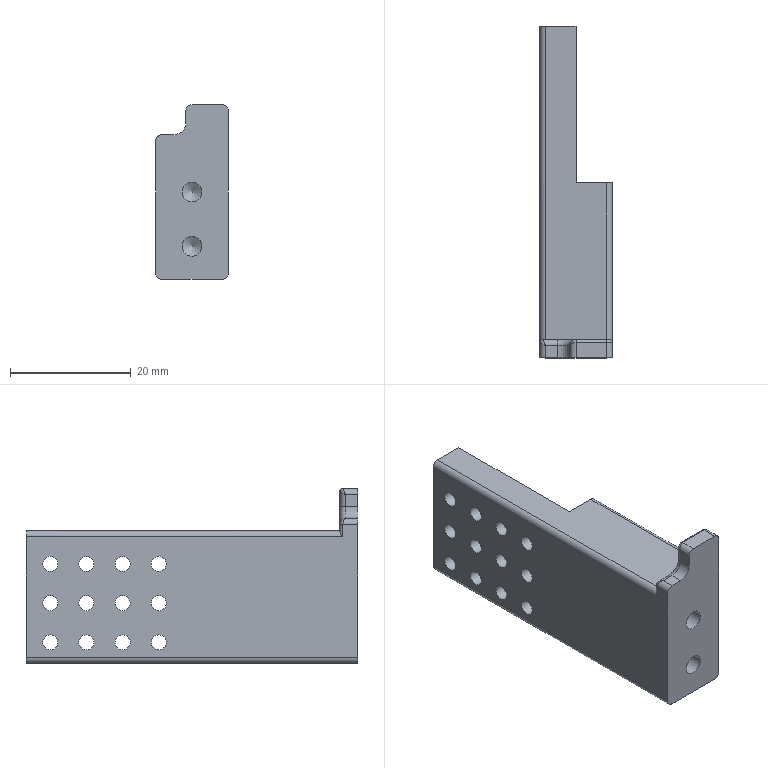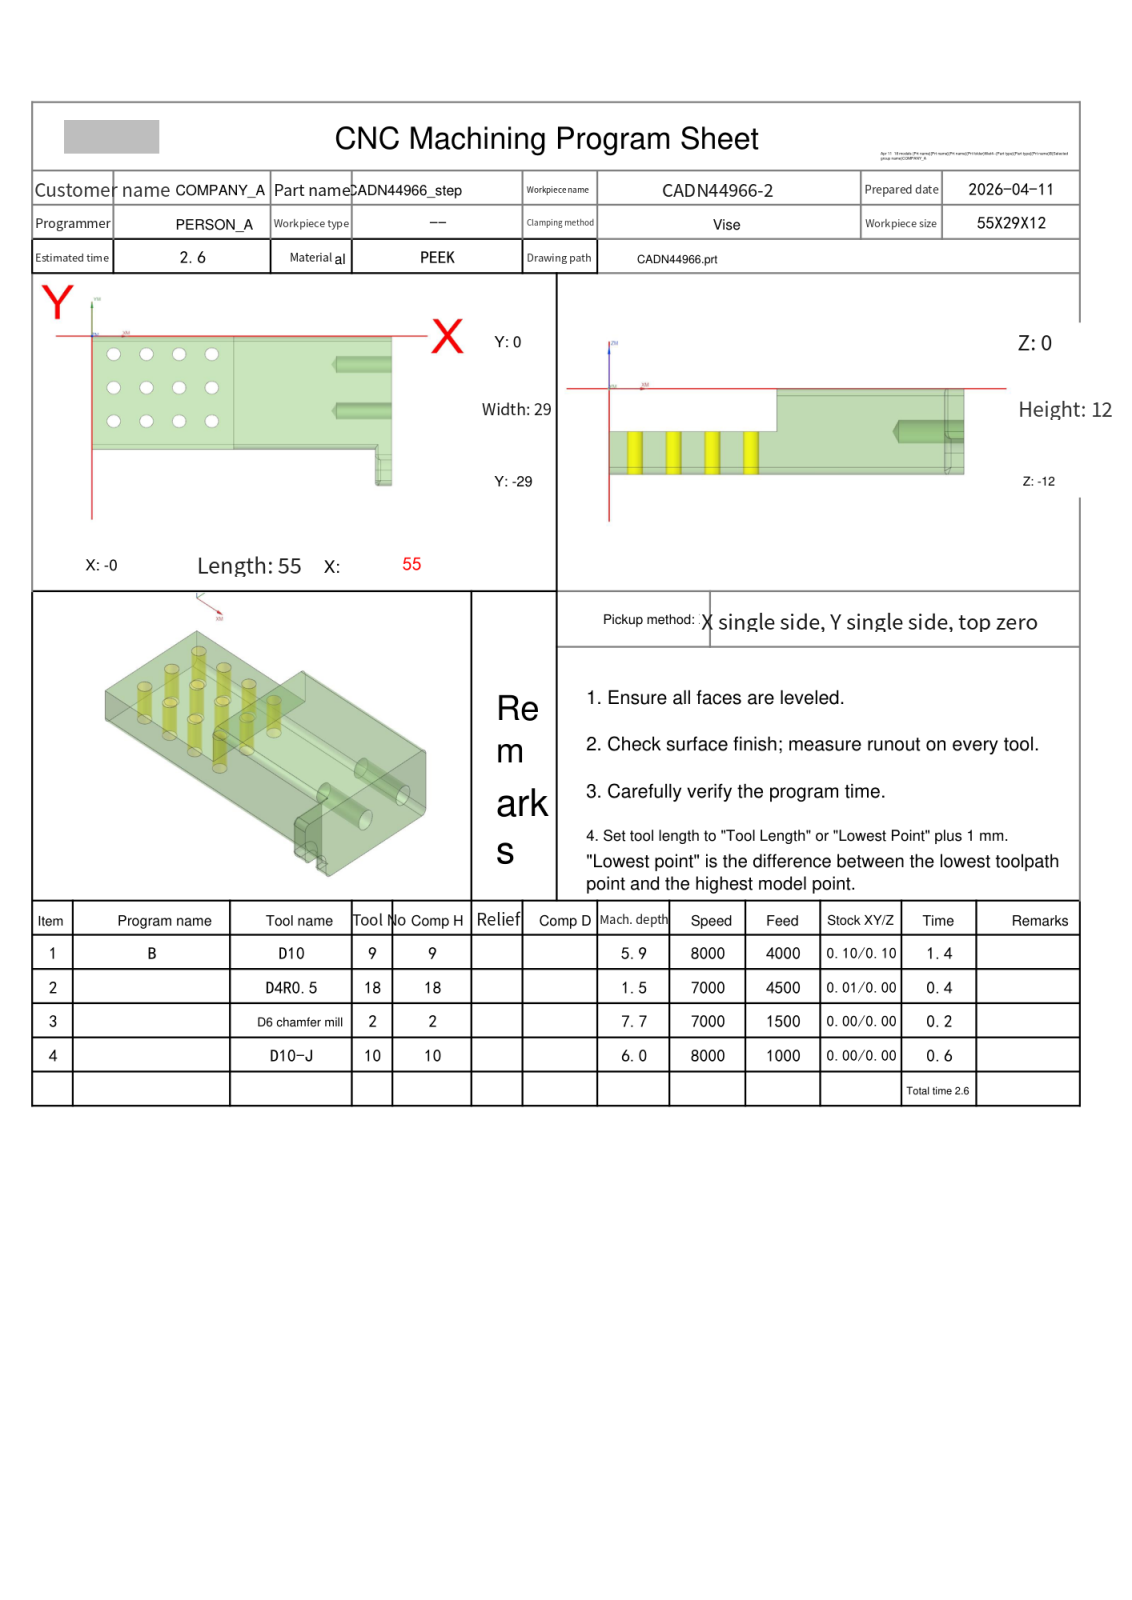NC program | NX | posted by the shop | part box 12 x 55 x 29 mm
Whole program:
%
O0001
(Machine time: 3.38 MIN)
(===Total Tool:4===)
(T9=D10     D=10.  R=0.   D-  H09 Z=-5.9  )
(T18=D4R0.5 D=4.   R=0.5  D-  H18 Z=-1.5  )
(T2=D6 chamfer mill   D=6.   R=0.   D-  H02 Z=-7.75 )
(T10=D10-J  D=10.  R=0.   D10 H10 Z=-6.   )
G80 G90 G17 G49 G40
G91 G28 Z0
M01
N1 T09 M06
(D10  D=10. R=0. H=09 ce=0.12 di=0.10)
G00 G90 G54 X56.095 Y-42.655 M03 S8000
G43 H09 Z20.
M08
Z2.1
G01 X56.077 Y-42.557 Z1.476 F4000.
X56.059 Y-42.458 Z1.228
X56.041 Y-42.36 Z1.046
X56.023 Y-42.262 Z.9
X56.005 Y-42.163 Z.777
X55.987 Y-42.065 Z.672
X55.969 Y-41.966 Z.58
X55.951 Y-41.868 Z.5
X55.933 Y-41.77 Z.43
X55.915 Y-41.671 Z.368
X55.897 Y-41.573 Z.314
X55.879 Y-41.475 Z.267
X55.861 Y-41.376 Z.227
X55.843 Y-41.278 Z.192
X55.825 Y-41.179 Z.164
X55.807 Y-41.081 Z.14
X55.789 Y-40.983 Z.123
X55.771 Y-40.884 Z.11
X55.753 Y-40.786 Z.103
X55.735 Y-40.688 Z.1
X55.321 Y-38.427
G03 X55.03 Y-38.057 I-.503 J-.096
X51.635 Y-37.525 I-3.395 J-10.561
G01 X51.626
G03 X43.205 Y-37.394 I-8.421 J-271.421
X41.31 Y-37.401 I0.0 J-271.551
G01 X-.989 Y-37.38
G02 X-7.02 Y-33.207 I.185 J6.712
X-8.224 Y-27.602 I15.006 J6.157
X-8.423 Y-18.028 I230.975 J9.574
X-8.4 Y-14.766 I231.173 J0.0
X-8.424 Y-8.547 I779.374 J6.218
X-8.363 Y1.242 I779.398 J0.0
X-4.159 Y7.045 I6.704 J-.433
X1.447 Y8.228 I6.146 J-15.246
X10.93 Y8.421 I9.482 J-232.83
X14.104 Y8.4 I0.0 J-233.023
G01 X55.963 Y8.381
G02 X62.132 Y3.982 I-.189 J-6.792
X63.262 Y-1.941 I-16.566 J-6.23
X63.415 Y-11.3 I-287.294 J-9.359
X63.4 Y-14.239 I-287.447 J0.0
X63.421 Y-20.5 I-911.502 J-6.261
X63.37 Y-30.142 I-911.524 J0.0
X58.582 Y-36.269 I-6.771 J.358
X54.233 Y-36.894 I-4.348 J14.824
X53.782 Y-36.887 I0.0 J15.449
G01 X40.41 Y-36.801
X.711 Y-36.78
G02 X-5.941 Y-32.409 I.315 J7.726
X-7.533 Y-26.233 I14.854 J7.123
X-7.815 Y-17.499 I135.288 J8.734
X-7.797 Y-15.319 I135.569 J0.0
X-7.818 Y-9.517 I806.989 J5.802
X-7.767 Y-.493 I807.009 J0.0
X-3.536 Y5.873 I7.677 J-.514
X2.628 Y7.52 I7.138 J-14.355
X10.532 Y7.802 I7.904 J-110.36
X11.921 Y7.794 I0.0 J-110.643
G01 X54.347 Y7.776
G02 X60.973 Y3.362 I-.367 J-7.73
X62.524 Y-2.643 I-14.759 J-7.014
X62.813 Y-11.23 I-127.375 J-8.587
X62.797 Y-13.256 I-127.664 J0.0
X62.821 Y-19.453 I-797.141 J-6.198
X62.77 Y-28.467 I-797.166 J0.0
X57.973 Y-35.016 I-7.438 J.417
X52.169 Y-36.124 I-6.063 J16.002
X43.452 Y-36.227 I-8.717 J371.111
X39.091 Y-36.201 I0.0 J371.213
G01 X2.331 Y-36.18
G02 X-5.254 Y-31.174 I.282 J8.677
X-6.907 Y-24.638 I16.474 J7.644
X-7.206 Y-15.973 I125.397 J8.665
X-7.194 Y-14.266 I125.696 J0.0
X-7.222 Y-9.478 I421.156 J4.788
X-7.154 Y-1.927 I421.184 J0.0
X-2.203 Y5.24 I8.641 J-.676
X4.331 Y6.904 I7.65 J-16.379
X13.376 Y7.212 I9.045 J-132.834
X15.424 Y7.196 I0.0 J-133.142
G01 X52.724 Y7.176
G02 X60.278 Y2.14 I-.328 J-8.674
X61.907 Y-4.341 I-16.543 J-7.604
X62.207 Y-13.032 I-125.802 J-8.692
X62.195 Y-14.773 I-126.102 J0.0
X62.213 Y-19.292 I-565.949 J-4.519
X62.16 Y-26.992 I-565.967 J0.0
X57.19 Y-34.019 I-8.205 J.533
X50.776 Y-35.435 I-7.008 J16.511
X42.826 Y-35.614 I-7.95 J176.599
X40.639 Y-35.6 I0.0 J176.778
G01 X3.819 Y-35.577
G02 X-4.639 Y-29.967 I.178 J9.45
X-6.299 Y-23.123 I18.212 J8.042
X-6.614 Y-13.443 I148.768 J9.68
X-6.596 Y-11.13 I149.082 J0.0
X-6.616 Y-8.452 I179.562 J2.678
X-6.542 Y-3.291 I179.582 J0.0
X-.926 Y4.659 I9.408 J-.688
X5.983 Y6.309 I8.053 J-18.428
X15.663 Y6.614 I9.68 J-153.667
X17.976 Y6.596 I0.0 J-153.971
G01 X51.076 Y6.58
G02 X59.696 Y.857 I-.08 J-9.474
X61.317 Y-6.064 I-18.725 J-8.037
X61.613 Y-15.695 I-156.564 J-9.631
X61.596 Y-17.997 I-156.86 J0.0
X61.621 Y-20.723 I-148.535 J-2.726
X61.535 Y-25.775 I-148.56 J0.0
X56.192 Y-33.235 I-8.923 J.749
X49.625 Y-34.766 I-7.505 J17.334
X40.929 Y-35.014 I-8.696 J152.605
X38.77 Y-34.999 I0.0 J152.853
G01 X5.37 Y-34.98
X5.274 Y-34.981
G02 X-4.078 Y-28.745 I0.0 J10.131
X-5.714 Y-21.518 I20.303 J8.395
X-6.007 Y-11.935 I156.398 J9.583
X-5.995 Y-9.945 I156.691 J0.0
X-6.021 Y-8.179 I60.045 J1.765
X-5.876 Y-4.009 I60.071 J0.0
X.061 Y3.988 I9.929 J-1.169
X7.149 Y5.685 I8.372 J-19.325
X16.964 Y6.011 I9.815 J-147.341
X19.141 Y5.995 I0.0 J-147.668
G01 X49.781 Y5.973
G02 X59.048 Y-.183 I-.024 J-10.089
X60.708 Y-7.401 I-19.977 J-8.395
X61.008 Y-17.015 I-154.105 J-9.614
X60.995 Y-19.035 I-154.405 J0.0
X61.02 Y-20.788 I-61.646 J-1.753
X60.886 Y-24.851 I-61.671 J0.0
X55.164 Y-32.537 I-9.504 J1.103
X48.362 Y-34.13 I-7.916 J18.473
X39.105 Y-34.414 I-9.257 J151.078
X36.908 Y-34.398 I0.0 J151.362
G01 X6.689 Y-34.378
X6.558
G02 X.003 Y-32.249 I0.0 J11.155
X-4.143 Y-25.856 I7.715 J9.543
X-5.262 Y-17.733 I32.465 J8.615
X-5.408 Y-10.962 I157.719 J6.771
X-5.321 Y-5.737 I157.864 J0.0
X1.122 Y3.387 I10.525 J-.596
X8.398 Y5.079 I8.628 J-20.619
X18.371 Y5.408 I9.973 J-150.721
X20.45 Y5.394 I0.0 J-151.051
G01 X48.15 Y5.381
G02 X48.363 Y5.383 I.213 J-11.468
X54.63 Y3.52 I0.0 J-11.47
X59.082 Y-2.937 I-7.106 J-9.662
X60.251 Y-10.99 I-30.991 J-8.611
X60.409 Y-17.99 I-155.203 J-7.
X60.322 Y-23.166 I-155.361 J0.0
X54.11 Y-31.898 I-10.124 J.626
X46.947 Y-33.524 I-8.306 J20.002
X37.515 Y-33.81 I-9.432 J155.667
X35.493 Y-33.797 I0.0 J155.953
G01 X7.973 Y-33.777
X7.814 Y-33.778
G02 X1.611 Y-32.108 I0.0 J12.357
X-3.247 Y-25.708 I6.554 J10.017
X-4.6 Y-17.688 I28.152 J8.874
X-4.788 Y-11.131 I113.955 J6.557
X-4.707 Y-6.833 I114.143 J0.0
X1.949 Y2.705 I10.937 J-.542
X9.39 Y4.457 I8.892 J-21.086
X19.292 Y4.803 I9.902 J-141.554
X21.082 Y4.792 I0.0 J-141.9
G01 X46.922 Y4.779
G02 X47.134 Y4.781 I.213 J-12.598
X53.199 Y3.225 I0.0 J-12.599
X58.253 Y-3.304 I-6.303 J-10.101
X59.602 Y-11.325 I-28.218 J-8.867
X59.786 Y-17.901 I-117.366 J-6.576
X59.716 Y-21.941 I-117.55 J0.0
X53.052 Y-31.294 I-10.628 J.522
X45.581 Y-32.925 I-8.623 J21.567
X36.008 Y-33.206 I-9.573 J162.578
X34.127 Y-33.196 I0.0 J162.859
G01 X9.127 Y-33.174
X8.963 Y-33.175
G02 X2.722 Y-31.621 I0.0 J13.307
X-2.558 Y-24.964 I6.285 J10.407
X-3.979 Y-16.834 I28.105 J9.104
X-4.165 Y-11.462 I77.747 J5.372
X-4.072 Y-7.66 I77.933 J0.0
X2.943 Y2.119 I11.3 J-.701
X10.693 Y3.87 I9.154 J-22.484
X21.08 Y4.207 I10.387 J-160.222
X23.165 Y4.193 I0.0 J-160.558
G01 X45.885 Y4.172
X46.04 Y4.173
G02 X52.183 Y2.676 I0.0 J-13.355
X57.521 Y-3.926 I-6.126 J-10.411
X58.969 Y-11.989 I-27.36 J-9.076
X59.164 Y-17.434 I-75.879 J-5.445
X59.073 Y-21.163 I-76.074 J0.0
X52.263 Y-30.595 I-10.967 J.743
X44.568 Y-32.305 I-8.929 J22.015
X34.018 Y-32.614 I-10.551 J179.427
X31.495 Y-32.597 I0.0 J179.737
G01 X10.335 Y-32.575
G02 X10.125 Y-32.576 I-.21 J14.524
X3.938 Y-31.193 I0.0 J14.526
X-1.75 Y-24.57 I5.776 J10.715
X-3.314 Y-16.653 I25.944 J9.239
X-3.528 Y-11.831 I54.412 J4.821
X-3.415 Y-8.321 I54.625 J0.0
X3.727 Y1.454 I11.556 J-.946
X11.47 Y3.241 I9.303 J-22.648
X22.25 Y3.608 I10.78 J-157.753
X24.481 Y3.593 I0.0 J-158.121
G01 X44.741 Y3.571
X44.92 Y3.572
G02 X51.129 Y2.16 I0.0 J-14.357
X56.819 Y-4.602 I-5.89 J-10.732
X58.333 Y-12.593 I-26.794 J-9.216
X58.525 Y-17.067 I-51.97 J-4.474
X58.416 Y-20.444 I-52.162 J0.0
X51.418 Y-29.94 I-11.262 J.973
X43.723 Y-31.676 I-9.091 J22.38
X33.432 Y-32.008 I-10.291 J159.374
X31.37 Y-31.994 I0.0 J159.705
G01 X11.59 Y-31.978
G02 X11.312 Y-31.98 I-.278 J16.163
X5.318 Y-30.828 I0.0 J16.166
X-1.016 Y-23.999 I5.124 J11.104
X-2.688 Y-15.922 I25.456 J9.481
X-2.879 Y-12.227 I35.588 J3.696
X-2.684 Y-8.496 I35.78 J0.0
X4.417 Y.76 I11.667 J-1.599
X12.265 Y2.616 I9.502 J-22.655
X22.413 Y2.995 I10.148 J-135.783
X23.835 Y2.987 I0.0 J-136.161
G01 X43.615 Y2.97
G02 X43.818 Y2.972 I.203 J-15.49
X49.979 Y1.694 I0.0 J-15.491
X56.047 Y-5.071 I-5.481 J-11.02
X57.7 Y-13.218 I-25.896 J-9.495
X57.876 Y-16.634 I-33.075 J-3.416
X57.675 Y-20.285 I-33.251 J0.0
X50.734 Y-29.23 I-11.386 J1.669
X43.06 Y-31.035 I-9.265 J22.175
X33.28 Y-31.395 I-9.78 J132.463
X31.969 Y-31.389 I0.0 J132.824
G01 X12.55 Y-31.374
G02 X12.289 Y-31.376 I-.261 J16.755
X6.101 Y-30.192 I0.0 J16.757
X-.368 Y-23.238 I5.207 J11.33
X-2.091 Y-14.803 I26.068 J9.719
X-2.215 Y-12.435 I22.511 J2.368
X-1.799 Y-8.115 I22.635 J0.0
X5.122 Y.082 I11.616 J-2.788
X12.841 Y1.972 I9.576 J-22.393
X23.581 Y2.4 I10.74 J-134.763
X25.369 Y2.388 I0.0 J-135.191
X32.366 Y2.415 I6.997 J-892.198
X43.109 Y2.351 I0.0 J-892.225
X49.708 Y.801 I-.021 J-14.912
X55.528 Y-6.162 I-6.257 J-11.144
X57.12 Y-14.622 I-27.671 J-9.586
X57.212 Y-16.505 I-19.266 J-1.882
X56.669 Y-21.056 I-19.357 J0.0
X49.888 Y-28.604 I-11.287 J3.32
X41.975 Y-30.437 I-9.485 J22.952
X31.605 Y-30.801 I-10.37 J147.233
X29.863 Y-30.791 I0.0 J147.597
X23.342 Y-30.822 I-6.521 J689.553
X12.604 Y-30.738 I0.0 J689.584
X5.803 Y-29.028 I.141 J14.943
X.143 Y-22.158 I6.624 J11.224
X-1.481 Y-12.87 I25.749 J9.288
X-1.335 Y-10.052 I27.373 J0.0
X5.685 Y-.655 I11.919 J-1.583
X13.677 Y1.358 I9.85 J-22.238
X24.523 Y1.798 I10.846 J-133.392
X26.265 Y1.787 I0.0 J-133.832
X32.297 Y1.812 I6.032 J-719.779
X42.264 Y1.743 I0.0 J-719.805
X49.081 Y.092 I-.07 J-15.193
X54.901 Y-6.953 I-6.51 J-11.303
X56.464 Y-15.953 I-25.138 J-9.
X56.339 Y-18.528 I-26.7 J0.0
X49.326 Y-27.858 I-11.718 J1.508
X41.617 Y-29.771 I-9.563 J22.047
X31.467 Y-30.191 I-10.15 J122.438
X30.229 Y-30.185 I0.0 J122.858
X23.681 Y-30.222 I-6.548 J578.841
X13.45 Y-30.131 I0.0 J578.878
X6.481 Y-28.357 I.175 J15.258
X.735 Y-21.297 I6.827 J11.425
X-.74 Y-13.15 I21.763 J8.147
X-.601 Y-10.617 I23.238 J0.0
X6.385 Y-1.323 I11.947 J-1.707
X14.189 Y.71 I9.877 J-21.92
X25.025 Y1.192 I10.836 J-121.547
X26.534 Y1.183 I0.0 J-122.029
X32.228 Y1.212 I5.694 J-545.285
X41.453 Y1.134 I0.0 J-545.315
X48.223 Y-.481 I-.146 J-15.608
X54.249 Y-7.66 I-6.445 J-11.529
X55.715 Y-15.624 I-20.904 J-7.964
X55.584 Y-18.041 I-22.369 J0.0
X48.773 Y-27.109 I-11.699 J1.694
X41.032 Y-29.128 I-9.732 J21.471
X30.321 Y-29.596 I-10.71 J122.211
X28.746 Y-29.586 I0.0 J122.679
X23.383 Y-29.618 I-5.363 J447.333
X14.307 Y-29.526 I0.0 J447.365
X7.431 Y-27.844 I.221 J15.803
X1.427 Y-20.711 I6.588 J11.639
X.035 Y-13.433 I18.327 J7.278
X.179 Y-11.05 I19.719 J0.0
X6.931 Y-2.064 I11.867 J-1.887
X14.829 Y.077 I10.038 J-21.395
X25.224 Y.577 I10.395 J-107.839
X26.093 Y.573 I0.0 J-108.339
X31.946 Y.609 I5.853 J-475.09
X40.552 Y.531 I0.0 J-475.126
X47.338 Y-1.034 I-.163 J-16.198
X53.574 Y-8.29 I-6.301 J-11.723
X54.93 Y-15.297 I-17.429 J-7.007
X54.774 Y-17.713 I-18.784 J0.0
X48.238 Y-26.352 I-11.597 J1.982
X40.519 Y-28.476 I-9.862 J20.749
X30.235 Y-28.98 I-10.284 J104.757
X29.316 Y-28.976 I0.0 J105.261
X23.757 Y-29.012 I-5.558 J426.474
X15.277 Y-28.928 I0.0 J426.51
X8.375 Y-27.33 I.191 J16.535
X2.071 Y-20.007 I6.35 J11.841
X.847 Y-13.755 I15.356 J6.252
X1.059 Y-11.116 I16.58 J0.0
X7.515 Y-2.787 I11.686 J-2.391
X15.51 Y-.55 I10.184 J-20.996
X26.013 Y-.026 I10.503 J-105.027
X26.832 Y-.029 I0.0 J-105.551
X31.974 Y.007 I5.142 J-361.178
X39.791 Y-.077 I0.0 J-361.214
X46.691 Y-1.705 I-.221 J-16.376
X52.972 Y-9.107 I-6.443 J-11.833
X54.105 Y-14.963 I-14.559 J-5.856
X53.874 Y-17.648 I-15.693 J0.0
X47.446 Y-25.725 I-11.465 J2.529
X39.617 Y-27.872 I-9.968 J20.996
X29.3 Y-28.377 I-10.317 J105.245
X28.474 Y-28.373 I0.0 J105.749
X23.655 Y-28.413 I-4.818 J290.722
X15.815 Y-28.308 I0.0 J290.762
X8.777 Y-26.537 I.344 J16.235
X2.512 Y-18.715 I6.814 J11.879
X1.695 Y-14.091 I12.673 J4.624
X2.261 Y-10.225 I13.49 J0.0
X8.508 Y-3.301 I11.371 J-3.98
X16.462 Y-1.143 I10.162 J-21.721
X27.002 Y-.627 I10.54 J-107.433
X27.785 Y-.63 I0.0 J-107.949
X32.096 Y-.59 I4.311 J-229.411
X39.363 Y-.705 I0.0 J-229.452
X46.505 Y-2.625 I-.41 J-15.772
X52.642 Y-10.795 I-7.197 J-11.797
X53.251 Y-14.623 I-11.728 J-3.828
X52.304 Y-19.364 I-12.337 J0.0
X46.002 Y-25.412 I-11.059 J5.217
X37.744 Y-27.375 I-10.063 J23.976
X26.542 Y-27.798 I-11.202 J148.115
X24.735 Y-27.787 I0.0 J148.538
X22.152 Y-27.817 I-2.583 J113.371
X15.619 Y-27.628 I0.0 J113.4
X7.864 Y-24.853 I.807 J14.481
X2.621 Y-14.122 I8.362 J10.731
X2.706 Y-12.609 I13.604 J0.0
X8.513 Y-4.35 I11.259 J-1.745
X16.187 Y-1.898 I10.246 J-18.832
X26.989 Y-1.238 I10.802 J-88.131
X27.68 Y-1.241 I0.0 J-88.79
X31.853 Y-1.193 I4.173 J-181.759
X38.778 Y-1.325 I0.0 J-181.807
X46.085 Y-3.422 I-.525 J-15.609
X52.296 Y-14.632 I-7.01 J-11.21
X52.249 Y-15.742 I-13.221 J0.0
X46.688 Y-24.003 I-10.998 J1.401
X39.038 Y-26.505 I-10.157 J18.111
X28.637 Y-27.156 I-10.401 J82.766
X28.205 Y-27.154 I0.0 J83.417
X23.919 Y-27.209 I-4.287 J167.666
X16.868 Y-27.061 I0.0 J167.72
X9.514 Y-24.891 I.625 J15.665
X3.578 Y-14.224 I6.616 J10.666
X3.587 Y-13.756 I12.552 J0.0
X8.91 Y-5.223 I10.909 J-.878
X16.463 Y-2.592 I10.284 J-17.365
X27.004 Y-1.86 I10.541 J-75.591
G01 X27.229 Y-1.861
G02 X31.539 Y-1.798 I4.311 J-149.275
X38.206 Y-1.947 I0.0 J-149.337
X45.645 Y-4.212 I-.646 J-15.474
X51.319 Y-14.532 I-6.549 J-10.32
G01 Y-14.588
G02 X46.291 Y-23.105 I-10.605 J.518
X38.823 Y-25.795 I-10.179 J16.546
X28.528 Y-26.536 I-10.295 J71.174
G01 X28.419
G02 X24.112 Y-26.598 I-4.306 J149.646
X17.741 Y-26.462 I0.0 J149.708
X10.362 Y-24.362 I.592 J16.095
X4.61 Y-15.13 I5.911 J10.091
X4.605 Y-14.809 I10.324 J.321
X9.15 Y-6.251 I10.329 J0.0
X16.464 Y-3.348 I10.285 J-15.246
X26.557 Y-2.493 I10.321 J-61.836
X31.239 Y-2.41 I4.682 J-131.427
X37.473 Y-2.557 I0.0 J-131.51
X44.865 Y-4.781 I-.69 J-15.689
X50.236 Y-13.328 I-5.91 J-9.676
X50.252 Y-13.894 I-9.975 J-.566
X46.083 Y-22.014 I-9.991 J0.0
X39.001 Y-24.992 I-10.126 J14.168
X29.095 Y-25.9 I-10.185 J56.645
X24.417 Y-25.989 I-4.678 J122.271
X18.18 Y-25.83 I0.0 J122.36
X10.841 Y-23.605 I.769 J15.753
X5.761 Y-15.889 I5.553 J9.185
X5.719 Y-14.984 I9.688 J.905
X9.556 Y-7.241 I9.731 J0.0
X16.643 Y-4.094 I10.222 J-13.467
X26.121 Y-3.131 I10.104 J-52.346
X30.973 Y-3.021 I4.852 J-106.47
X37.036 Y-3.193 I0.0 J-106.581
X44.441 Y-5.584 I-.857 J-15.316
X49.076 Y-12.918 I-5.526 J-8.625
X49.107 Y-13.679 I-9.46 J-.761
X45.366 Y-21.229 I-9.491 J0.0
X38.172 Y-24.374 I-10.139 J13.392
X28.208 Y-25.298 I-10.224 J56.087
X24.423 Y-25.378 I-3.786 J89.619
X18.494 Y-25.182 I0.0 J89.699
X11.07 Y-22.663 I.956 J15.018
X6.896 Y-15.243 I5.25 J7.838
X10.802 Y-7.623 I9.466 J-.042
X17.763 Y-4.648 I9.997 J-13.759
X27.725 Y-3.711 I10.288 J-55.924
X31.086 Y-3.634 I3.361 J-73.788
X36.838 Y-3.859 I0.0 J-73.864
X44.188 Y-6.538 I-1.1 J-14.437
X47.88 Y-13.729 I-5.157 J-7.191
X47.866 Y-14.216 I-8.849 J0.0
X43.676 Y-21.148 I-9.439 J.972
X36.624 Y-23.896 I-9.82 J14.779
X26.375 Y-24.718 I-10.248 J63.512
G01 X26.347
G02 X24.069 Y-24.766 I-2.278 J54.386
X18.2 Y-24.448 I0.0 J54.433
X11.195 Y-21.556 I1.425 J13.38
X8.2 Y-15.202 I5.243 J6.354
X10.311 Y-9.694 I8.238 J0.0
X16.721 Y-5.761 I9.93 J-8.992
X25.482 Y-4.439 I9.899 J-35.905
X30.58 Y-4.263 I5.098 J-74.115
X36.033 Y-4.464 I0.0 J-74.29
X42.899 Y-6.769 I-1.045 J-14.494
X46.535 Y-13.466 I-4.35 J-6.697
X44.515 Y-18.775 I-7.986 J0.0
X38.267 Y-22.651 I-9.714 J8.686
X29.507 Y-23.972 I-9.796 J35.236
X24.902 Y-24.127 I-4.605 J68.466
X19.676 Y-23.928 I0.0 J68.621
X13.223 Y-21.863 I1.048 J14.388
X9.594 Y-15.358 I4.016 J6.505
X11.228 Y-10.635 I7.645 J0.0
X17.267 Y-6.517 I9.61 J-7.606
X25.522 Y-5.095 I9.618 J-31.15
X30.428 Y-4.894 I4.905 J-59.872
X35.71 Y-5.127 I0.0 J-60.072
X41.889 Y-7.251 I-1.156 J-13.41
X45.084 Y-13.311 I-4.148 J-6.059
X43.669 Y-17.644 I-7.343 J0.0
X37.96 Y-21.789 I-9.35 J6.875
X30.024 Y-23.275 I-9.376 J28.13
X25.091 Y-23.494 I-4.933 J55.486
X19.898 Y-23.251 I0.0 J55.704
X14.21 Y-21.329 I1.149 J12.775
X11.127 Y-15.506 I3.957 J5.822
X12.299 Y-11.617 I7.04 J0.0
X17.92 Y-7.289 I9.235 J-6.179
X25.726 Y-5.754 I9.306 J-26.718
X30.339 Y-5.536 I4.613 J-48.79
X35.311 Y-5.789 I0.0 J-49.007
X40.695 Y-7.682 I-1.108 J-11.755
X43.477 Y-13.151 I-3.985 J-5.469
X42.452 Y-16.731 I-6.767 J0.0
X37.111 Y-21.055 I-8.963 J5.611
X29.5 Y-22.631 I-9.084 J24.695
X25.14 Y-22.848 I-4.359 J43.676
X20.158 Y-22.565 I0.0 J43.893
X15.365 Y-20.803 I1.07 J10.313
X12.831 Y-15.662 I3.949 J5.142
X13.658 Y-12.494 I6.483 J0.0
X18.767 Y-8.057 I8.77 J-4.94
X26.414 Y-6.39 I9.048 J-23.133
X30.304 Y-6.19 I3.889 J-37.575
X35.154 Y-6.502 I0.0 J-37.776
X39.588 Y-8.336 I-.992 J-8.677
X41.666 Y-13.003 I-4.201 J-4.667
X40.87 Y-16.063 I-6.279 J0.0
X35.77 Y-20.45 I-8.59 J4.829
X28.164 Y-22.039 I-8.791 J23.075
X25.074 Y-22.188 I-3.09 J32.073
X20.327 Y-21.836 I0.0 J32.222
X15.966 Y-19.433 I.88 J6.755
X14.782 Y-15.774 I5.063 J3.659
X15.82 Y-12.326 I6.246 J0.0
X21.02 Y-8.326 I8.447 J-5.601
X29.205 Y-6.908 I8.602 J-25.313
X30.715 Y-6.855 I1.51 J-21.551
X35.347 Y-7.357 I0.0 J-21.604
X39.596 Y-12.832 I-1.402 J-5.475
X39.218 Y-14.864 I-5.651 J0.0
X34.853 Y-19.537 I-8. J3.098
X27.858 Y-21.332 I-8.251 J17.619
X25.071 Y-21.497 I-2.787 J23.46
X21.221 Y-21.181 I0.0 J23.625
X17.02 Y-15.977 I1.124 J5.205
X17.237 Y-14.472 I5.325 J0.0
X21.37 Y-9.557 I7.727 J-2.302
X28.336 Y-7.701 I7.982 J-15.961
X30.404 Y-7.58 I2.068 J-17.628
X33.358 Y-7.828 I0.0 J-17.749
X37.103 Y-12.668 I-1.255 J-4.841
X36.985 Y-13.75 I-5.001 J0.0
X33.239 Y-18.731 I-7.361 J1.637
X26.427 Y-20.656 I-7.608 J13.904
X25.119 Y-20.742 I-1.308 J9.892
X23.086 Y-20.533 I0.0 J9.978
X19.857 Y-16.113 I1.41 J4.419
X19.899 Y-15.491 I4.639 J0.0
X23.264 Y-10.399 I6.96 J-.942
X30.038 Y-8.483 I6.773 J-11.014
G01 X30.17 Y-8.484
G02 X33.629 Y-12.159 I-.536 J-3.969
X33.646 Y-12.625 I-6.131 J-.466
X31.226 Y-17.515 I-6.149 J0.0
X28.113 Y-19.132 I-4.97 J5.761
X24.81 Y-17.45 I.056 J4.193
G01 X24.744 Y-17.375 Z.103
X24.678 Y-17.3 Z.11
X24.612 Y-17.225 Z.123
X24.546 Y-17.15 Z.14
X24.48 Y-17.075 Z.164
X24.414 Y-17. Z.192
X24.348 Y-16.925 Z.227
X24.281 Y-16.85 Z.267
X24.215 Y-16.775 Z.314
X24.149 Y-16.7 Z.368
X24.083 Y-16.625 Z.43
X24.017 Y-16.55 Z.5
X23.951 Y-16.475 Z.58
X23.885 Y-16.4 Z.672
X23.819 Y-16.325 Z.777
X23.752 Y-16.25 Z.9
X23.686 Y-16.175 Z1.046
X23.62 Y-16.1 Z1.228
X23.554 Y-16.025 Z1.476
X23.488 Y-15.95 Z2.1
G00 Z20.
G00 G90 X-1.6 Y8. M03 S8000
Z12.8
Z.91
G01 Z-.59 F4000.
Y4.9
Y-25.9
G03 X-.6 Y-26.9 I1. J0.0
G01 X4.9
G03 X5.9 Y-25.9 I0.0 J1.
G01 Y3.9
G02 X6.9 Y4.9 I1. J0.0
G01 X12.4
G02 X13.4 Y3.9 I0.0 J-1.
G01 Y-26.044
G03 X14.246 Y-27.032 I1. J0.0
G01 X19.746 Y-27.888
X19.9 Y-27.9
G03 X20.9 Y-26.9 I0.0 J1.
G01 Y4.9
Y8.012
Z.91
G00 X-1.6 Y8.
Z.32
G01 Z-1.18
Y4.9
Y-25.9
G03 X-.6 Y-26.9 I1. J0.0
G01 X4.9
G03 X5.9 Y-25.9 I0.0 J1.
G01 Y3.9
G02 X6.9 Y4.9 I1. J0.0
G01 X12.4
G02 X13.4 Y3.9 I0.0 J-1.
G01 Y-26.044
G03 X14.246 Y-27.032 I1. J0.0
G01 X19.746 Y-27.888
X19.9 Y-27.9
G03 X20.9 Y-26.9 I0.0 J1.
G01 Y4.9
Y8.1
Z.32
G00 X-1.6 Y8.
Z-.27
G01 Z-1.77
Y4.9
Y-25.9
G03 X-.6 Y-26.9 I1. J0.0
G01 X4.9
G03 X5.9 Y-25.9 I0.0 J1.
G01 Y3.9
G02 X6.9 Y4.9 I1. J0.0
G01 X12.4
G02 X13.4 Y3.9 I0.0 J-1.
G01 Y-26.044
G03 X14.246 Y-27.032 I1. J0.0
G01 X19.746 Y-27.888
X19.9 Y-27.9
G03 X20.9 Y-26.9 I0.0 J1.
G01 Y4.9
Y8.1
Z-.27
G00 X-1.6 Y8.
Z-.86
G01 Z-2.36
Y4.9
Y-25.9
G03 X-.6 Y-26.9 I1. J0.0
G01 X4.9
G03 X5.9 Y-25.9 I0.0 J1.
G01 Y3.9
G02 X6.9 Y4.9 I1. J0.0
G01 X12.4
G02 X13.4 Y3.9 I0.0 J-1.
G01 Y-26.044
G03 X14.246 Y-27.032 I1. J0.0
G01 X19.746 Y-27.888
X19.9 Y-27.9
G03 X20.9 Y-26.9 I0.0 J1.
G01 Y4.9
Y8.1
Z-.86
G00 X-1.6 Y8.
Z-1.45
G01 Z-2.95
Y4.9
Y-25.9
G03 X-.6 Y-26.9 I1. J0.0
G01 X4.9
G03 X5.9 Y-25.9 I0.0 J1.
G01 Y3.9
G02 X6.9 Y4.9 I1. J0.0
G01 X12.4
G02 X13.4 Y3.9 I0.0 J-1.
G01 Y-26.044
G03 X14.246 Y-27.032 I1. J0.0
G01 X19.746 Y-27.888
X19.9 Y-27.9
G03 X20.9 Y-26.9 I0.0 J1.
G01 Y4.9
Y8.1
Z-1.45
G00 X-1.6 Y8.
Z-2.04
G01 Z-3.54
Y4.9
Y-25.9
G03 X-.6 Y-26.9 I1. J0.0
G01 X4.9
G03 X5.9 Y-25.9 I0.0 J1.
G01 Y3.9
G02 X6.9 Y4.9 I1. J0.0
G01 X12.4
G02 X13.4 Y3.9 I0.0 J-1.
G01 Y-26.044
G03 X14.246 Y-27.032 I1. J0.0
G01 X19.746 Y-27.888
X19.9 Y-27.9
G03 X20.9 Y-26.9 I0.0 J1.
G01 Y4.9
Y8.1
Z-2.04
G00 X-1.6 Y8.
Z-2.63
G01 Z-4.13
Y4.9
Y-25.9
G03 X-.6 Y-26.9 I1. J0.0
G01 X4.9
G03 X5.9 Y-25.9 I0.0 J1.
G01 Y3.9
G02 X6.9 Y4.9 I1. J0.0
G01 X12.4
G02 X13.4 Y3.9 I0.0 J-1.
G01 Y-26.044
G03 X14.246 Y-27.032 I1. J0.0
G01 X19.746 Y-27.888
X19.9 Y-27.9
G03 X20.9 Y-26.9 I0.0 J1.
G01 Y4.9
Y8.1
Z-2.63
G00 X-1.6 Y8.
Z-3.22
G01 Z-4.72
Y4.9
Y-25.9
G03 X-.6 Y-26.9 I1. J0.0
G01 X4.9
G03 X5.9 Y-25.9 I0.0 J1.
G01 Y3.9
G02 X6.9 Y4.9 I1. J0.0
G01 X12.4
G02 X13.4 Y3.9 I0.0 J-1.
G01 Y-26.044
G03 X14.246 Y-27.032 I1. J0.0
G01 X19.746 Y-27.888
X19.9 Y-27.9
G03 X20.9 Y-26.9 I0.0 J1.
G01 Y4.9
Y8.1
Z-3.22
G00 X-1.6 Y8.
Z-3.81
G01 Z-5.31
Y4.9
Y-25.9
G03 X-.6 Y-26.9 I1. J0.0
G01 X4.9
G03 X5.9 Y-25.9 I0.0 J1.
G01 Y3.9
G02 X6.9 Y4.9 I1. J0.0
G01 X12.4
G02 X13.4 Y3.9 I0.0 J-1.
G01 Y-26.044
G03 X14.246 Y-27.032 I1. J0.0
G01 X19.746 Y-27.888
X19.9 Y-27.9
G03 X20.9 Y-26.9 I0.0 J1.
G01 Y4.9
Y8.1
Z-3.81
G00 X-1.6 Y8.
Z-4.4
G01 Z-5.9
Y4.9
Y-25.9
G03 X-.6 Y-26.9 I1. J0.0
G01 X4.9
G03 X5.9 Y-25.9 I0.0 J1.
G01 Y3.9
G02 X6.9 Y4.9 I1. J0.0
G01 X12.4
G02 X13.4 Y3.9 I0.0 J-1.
G01 Y-26.044
G03 X14.246 Y-27.032 I1. J0.0
G01 X19.746 Y-27.888
X19.9 Y-27.9
G03 X20.9 Y-26.9 I0.0 J1.
G01 Y4.9
Y8.1
Z-4.4
G00 Z12.8
G91 G28 Z0.0
M05
M09
G91 G28 Z0.0
M01
N2 T18 M06
(D4R0.5  D=4. R=0.5 H=18 ce=0.01 di=0.00)
G00 G90 G54 X59.14 Y-29.93 M03 S7000
G43 H18 Z12.8
M08
Z.488
G01 Z-.012 F4500.
X56.1 Y-29.621
G03 X55.773 Y-29.604 I-.327 J-3.212
X55. Y-29.698 I0.0 J-3.229
G01 X52.5
G02 X50.837 Y-28. I.117 J1.778
G01 Y-22.698
X26.
X25.114 Y-22.613
X24.899 Y-22.611
Y-22.653 Z-.019
Y-22.666 Z-.026
X26. Y-22.788
X50.764
Y-28.
G03 X52.5 Y-29.788 I1.851 J.061
G01 X55.
G02 X55.722 Y-29.672 I.722 J-2.201
X56.097 Y-29.703 I0.0 J-2.316
G01 Y-29.741 Z-.034
X56.098 Y-29.771 Z-.043
G03 X55.784 Y-29.754 I-.313 J-2.782
X55. Y-29.866 I0.0 J-2.799
G01 X52.5
G02 X50.7 Y-28. I.085 J1.882
G01 Y-22.866
X26.
X25.114 Y-22.741
X24.9 Y-22.733
Y-22.793 Z-.054
Y-22.817 Z-.064
X26. Y-22.945
X50.637
Y-28.
Y-28.041
G03 X52.5 Y-29.945 I1.904 J0.0
G01 X55.
G02 X55.883 Y-29.845 I.883 J-3.841
X56.1 Y-29.851 I0.0 J-3.941
G01 Y-29.894 Z-.077
Y-29.916 Z-.09
X55.963 Y-29.914
G03 X55. Y-30.023 I0.0 J-4.302
G01 X52.5
G02 X50.575 Y-28.013 I.086 J2.01
G01 Y-28.
Y-23.023
X26.
G03 X24.9 Y-22.901 I-1.263 J-6.374
G01 Y-22.947 Z-.106
Y-22.978 Z-.122
G02 X26. Y-23.103 I-.121 J-5.959
G01 X50.511
Y-28.
Y-28.032
G03 X52.5 Y-30.103 I2.073 J0.0
G01 X55.
G02 X56.071 Y-29.99 I1.071 J-5.022
G01 X56.1
Y-30.046 Z-.141
Y-30.078 Z-.16
X55.55 Y-30.085
G02 X55.012 Y-30.184 I-.538 J1.416
G01 X55.
X52.5
G02 X50.447 Y-28.04 I.093 J2.144
G01 X50.448 Y-28.
Y-23.184
X26.
G02 X25.396 Y-23.075 I.007 J1.77
G01 X24.9 Y-23.068
Y-23.122 Z-.181
Y-23.168 Z-.203
X24.96 Y-23.167
G02 X26. Y-23.263 I0.0 J-5.69
G01 X50.386
Y-28.
G03 X50.477 Y-28.636 I3.529 J.181
X52.5 Y-30.263 I2.088 J.524
G01 X55.
G02 X56.03 Y-30.171 I1.03 J-5.688
G01 X56.1
Y-30.218 Z-.228
Y-30.262 Z-.252
X55.995 Y-30.261
G03 X55. Y-30.342 I0.0 J-6.155
G01 X52.5
G02 X50.695 Y-29.303 I.049 J2.172
G01 X50.594 Y-29.107
G02 X50.326 Y-28.003 I2.143 J1.104
G01 Y-23.342
X26.
G03 X24.976 Y-23.257 I-1.024 J-6.125
G01 X24.9 Y-23.258
Y-23.301 Z-.28
Y-23.339 Z-.307
X25.004 Y-23.338
G02 X26. Y-23.419 I0.0 J-6.159
G01 X50.269
Y-28.
G03 X50.382 Y-28.744 I3.208 J.105
X52.5 Y-30.419 I2.178 J.577
G01 X55.
X55.409 Y-30.37
X55.479 Y-30.351
X55.55 Y-30.34
X56.1
Y-30.38 Z-.337
Y-30.419 Z-.368
X55.55
G02 X55. Y-30.494 I-.696 J3.064
G01 X52.5
G02 X50.321 Y-28.744 I.066 J2.314
X50.215 Y-28. I3.74 J.909
G01 Y-23.494
X26.
G03 X25.027 Y-23.417 I-.973 J-6.121
G01 X24.9 Y-23.418
Y-23.462 Z-.4
Y-23.495 Z-.433
X25.066 Y-23.493
G02 X26. Y-23.565 I0.0 J-6.084
G01 X50.166
Y-28.
G03 X50.477 Y-29.301 I2.995 J.029
X52.5 Y-30.565 I2.07 J1.061
G01 X55.
G03 X55.55 Y-30.497 I-.126 J3.296
G01 X56.1
Y-30.536 Z-.469
Y-30.574 Z-.504
G03 X55.871 Y-30.57 I-.229 J-6.159
X55. Y-30.632 I0.0 J-6.163
G01 X52.5
G02 X50.462 Y-29.386 I.038 J2.352
X50.151 Y-28.337 I2.414 J1.286
G01 X50.122 Y-28.
Y-23.632
X26.
G03 X25.088 Y-23.572 I-.912 J-6.901
G01 X24.9 Y-23.574
Y-23.604 Z-.542
Y-23.633 Z-.58
X25.078 Y-23.63
G02 X26. Y-23.695 I0.0 J-6.636
G01 X50.083
Y-28.
Y-28.012
G03 X50.477 Y-29.517 I3.07 J0.0
X52.5 Y-30.695 I2.064 J1.22
G01 X55.
X55.268 Y-30.672
X55.409 Y-30.644
G02 X55.825 Y-30.624 I.416 J-4.245
X56.1 Y-30.633 I0.0 J-4.265
G01 Y-30.664 Z-.619
Y-30.695 Z-.659
X55.55
X55.457 Y-30.701
G02 X55. Y-30.752 I-.645 J3.719
G01 X52.5
X52.45 Y-30.75
X52.168 Y-30.725
X52.157 Y-30.719
X52.054 Y-30.707
X52.02 Y-30.701
X51.886 Y-30.664
X51.604 Y-30.568
X51.323 Y-30.43
X51.041 Y-30.238
G02 X50.419 Y-29.495 I1.48 J1.871
X50.076 Y-28.368 I2.297 J1.314
G01 X50.05 Y-28.
Y-23.752
X26.
G03 X25.058 Y-23.692 I-.942 J-7.347
G01 X24.9 Y-23.694
Y-23.727 Z-.701
Y-23.753 Z-.743
X25.059 Y-23.751
G02 X26. Y-23.805 I0.0 J-8.326
G01 X50.024
Y-28.
G03 X50.111 Y-28.815 I4.308 J.052
X51.323 Y-30.491 I2.528 J.551
X52.5 Y-30.805 I1.238 J2.277
G01 X55.
G02 X55.856 Y-30.751 I.856 J-6.78
X56.1 Y-30.755 I0.0 J-6.833
G01 Y-30.783 Z-.786
Y-30.801 Z-.83
X55.55 Y-30.803
X55.456 Y-30.808
X55. Y-30.852
X52.5
G02 X50.195 Y-29.196 I.034 J2.479
X50.004 Y-28.053 I3.323 J1.143
G01 X50.005 Y-28.
Y-23.852
X26.
G03 X25.087 Y-23.801 I-.913 J-8.156
G01 X24.9 Y-23.803
Y-23.826 Z-.875
Y-23.846 Z-.921
G02 X25.102 Y-23.844 I.202 J-8.147
X26. Y-23.894 I0.0 J-8.15
G01 X49.993
Y-28.
X49.997 Y-28.01
X50.01 Y-28.376
G03 X50.269 Y-29.454 I2.806 J.104
X52.5 Y-30.894 I2.255 J1.046
G01 X55.
G02 X55.948 Y-30.841 I.948 J-8.566
G01 X56.1 Y-30.843
Y-30.863 Z-.967
X56.101 Y-30.883 Z-1.014
X56.04 Y-30.882
G03 X55. Y-30.929 I0.0 J-11.618
G01 X52.5
G02 X50.09 Y-29.024 I.024 J2.507
X49.99 Y-28.185 I3.468 J.839
G01 Y-23.929
X26.
G03 X25.145 Y-23.885 I-.855 J-8.301
X24.901 Y-23.889 I0.0 J-8.345
G01 Y-23.909 Z-1.061
Y-23.927 Z-1.109
G02 X25.184 Y-23.923 I.283 J-9.431
X26. Y-23.958 I0.0 J-9.435
G01 X49.99
Y-28.185
X49.999 Y-28.464
G03 X52.5 Y-30.958 I2.529 J.035
G01 X55.
G02 X55.978 Y-30.919 I.978 J-12.205
G01 X56.1 Y-30.92
Y-30.936 Z-1.158
Y-30.949 Z-1.207
X56.001 Y-30.948
G03 X55. Y-30.981 I0.0 J-15.409
G01 X52.494
G02 X51.313 Y-30.673 I0.0 J2.419
G01 X51.164 Y-30.59
G02 X50.036 Y-28.889 I1.365 J2.129
X49.99 Y-28.345 I3.174 J.543
G01 Y-23.981
X26.
G03 X25.196 Y-23.948 I-.804 J-9.812
X24.9 Y-23.953 I0.0 J-9.845
G01 Y-23.974 Z-1.255
Y-23.978 Z-1.304
G02 X25.198 Y-23.975 I.298 J-14.618
X26. Y-23.997 I0.0 J-14.621
G01 X49.989
X49.99 Y-24.01
Y-28.464
G03 X50.056 Y-29.024 I3.06 J.078
X51.604 Y-30.829 I2.454 J.539
X52.5 Y-30.997 I.972 J2.701
G01 X55.
G02 X56.029 Y-30.978 I1.029 J-27.778
G01 X56.1
X56.103 Y-30.989 Z-1.353
X56.105 Y-30.997 Z-1.402
X55. Y-31.007
X52.5
G02 X50.61 Y-30.142 I.036 J2.577
X49.99 Y-28.474 I1.935 J1.668
G01 Y-28.464
Y-24.007
X26.
X25.959 Y-24.003
X24.91 Y-23.998
X24.927 Y-24.009 Z-1.5
X49.99 Y-24.01
Y-28.464
Y-28.498
G03 X52.45 Y-31.009 I2.512 J0.0
G01 X56.105 Y-31.01
G00 Z12.8
G00 G90 X21.675 Y.602 M03 S7000
Z12.8
Z.488
G01 Z-.012 F4500.
X24.9 Y.613
X25.114
X26. Y.7
X55.
X56.1 Y.611
Y.657 Z-.02
Y.676 Z-.029
X55. Y.801
X26.
X25.114 Y.684
X24.9
Y.753 Z-.038
Y.769 Z-.048
X26. Y.888
X55.
X56.1 Y.753
Y.815 Z-.06
Y.844 Z-.072
X55. Y.968
X26.
X25.114 Y.869
X24.9
Y.912 Z-.085
Y.934 Z-.099
G03 X26. Y1.047 I-.077 J6.148
G01 X55.
G03 X56.1 Y.921 I1.495 J8.169
G01 Y.968 Z-.116
Y1.003 Z-.133
G02 X55. Y1.128 I.308 J7.637
G01 X26.
G02 X24.9 Y1.013 I-1.17 J5.874
G01 Y1.068 Z-.153
Y1.105 Z-.172
X25.114
X26. Y1.208
X55.
G03 X56.1 Y1.099 I1.451 J9.036
G01 Y1.153 Z-.195
Y1.194 Z-.217
G02 X55. Y1.287 I.105 J7.798
G01 X26.
G02 X24.9 Y1.196 I-1.133 J6.959
G01 Y1.243 Z-.243
Y1.288 Z-.268
X24.955
G03 X26. Y1.366 I0.0 J7.055
G01 X55.
G03 X56.058 Y1.289 I1.058 J7.259
G01 X56.1
Y1.326 Z-.297
Y1.363 Z-.325
G02 X55. Y1.442 I.067 J8.632
G01 X26.
X25.959 Y1.44
X25.396 Y1.37
X24.9 Y1.362
Y1.404 Z-.356
Y1.441 Z-.387
X24.953
G03 X26. Y1.516 I0.0 J7.419
G01 X55.
G03 X56.048 Y1.442 I1.048 J7.451
G01 X56.1
Y1.485 Z-.421
Y1.521 Z-.454
X56.097
G02 X55. Y1.585 I0.0 J9.35
G01 X26.
G02 X24.906 Y1.52 I-1.094 J9.08
G01 X24.9
Y1.557 Z-.491
Y1.591 Z-.527
X25.027 Y1.59
G03 X26. Y1.651 I0.0 J7.777
G01 X55.
G03 X55.985 Y1.591 I.985 J8.051
G01 X56.1 Y1.592
Y1.623 Z-.565
Y1.652 Z-.604
X56.011 Y1.651
G02 X55. Y1.713 I0.0 J8.325
G01 X26.
G02 X24.941 Y1.651 I-1.059 J9.008
G01 X24.9
Y1.683 Z-.644
Y1.713 Z-.685
X24.999 Y1.712
G03 X26. Y1.769 I0.0 J8.836
G01 X55.
G03 X56.015 Y1.713 I1.015 J9.199
G01 X56.1 Y1.714
Y1.741 Z-.727
Y1.774 Z-.77
X55.935 Y1.772
G02 X55. Y1.82 I0.0 J9.151
G01 X26.
G02 X25.016 Y1.772 I-.984 J10.035
G01 X24.9 Y1.773
Y1.792 Z-.814
Y1.814 Z-.858
X24.963 Y1.813
G03 X26. Y1.866 I0.0 J10.305
G01 X55.
G03 X55.969 Y1.816 I.969 J9.44
G01 X56.1 Y1.817
Y1.839 Z-.904
Y1.86 Z-.949
X55.91 Y1.858
G02 X55. Y1.905 I0.0 J8.84
G01 X26.
G02 X24.925 Y1.854 I-1.075 J11.247
G01 X24.9
Y1.875 Z-.996
X24.899 Y1.894 Z-1.043
G03 X26. Y1.939 I-.172 J17.672
G01 X55.
G03 X55.907 Y1.902 I.907 J11.149
G01 X56.1 Y1.904
Y1.919 Z-1.091
Y1.935 Z-1.14
X55.922 Y1.934
G02 X55. Y1.966 I0.0 J13.255
G01 X26.
G02 X24.9 Y1.928 I-1.294 J21.715
G01 Y1.944 Z-1.185
Y1.955 Z-1.23
G03 X26. Y1.985 I-.227 J27.759
G01 X55.
G03 X55.9 Y1.959 I.9 J15.298
G01 X56.1 Y1.96
X56.103 Y1.977 Z-1.275
X56.105 Y1.985 Z-1.32
G02 X55.84 Y1.984 I-.265 J23.076
X55. Y1.999 I0.0 J23.078
G01 X26.
X25.959 Y1.994
X24.9 Y1.981
X24.913 Y1.998 Z-1.41
X25.959 Y2.003
X26. Y2.007
X55.
X56.105 Y1.999
Y2.008 Z-1.455
Y2.01 Z-1.5
X24.928 Y2.009
G00 Z12.8
G91 G28 Z0.0
M05
M09
G91 G28 Z0.0
M01
N3 T02 M06
(D6 chamfer mill  D=6. R=0. H=02 ce=0.00 di=0.00)
G00 G90 G54 X25.273 Y-21.386 M03 S6500
G43 H02 Z20.
M08
Z.627
G01 Z-.7 F1500.
G03 X25.473 Y-21.1 I-1.532 J1.286
G01 X25.503 Y-21.054
X25.5 Y-21.
Y-1.
X25.503 Y-.946
X25.473 Y-.9
G03 X25.273 Y-.614 I-1.732 J-1.
G01 Z.627
G00 Z10.
X55.727
Z.627
G01 Z-.7
G03 X55.527 Y-.9 I1.532 J-1.286
G01 X55.497 Y-.946
X55.5 Y-1.
Y-28.
X55.497 Y-28.054
X55.527 Y-28.1
G03 X55.727 Y-28.386 I1.732 J1.
G01 Z.627
G00 Z10.
X22.827 Y-22.545
Z-2.059
G01 Z-6.7
X22.77 Y-22.505
X22.75 Y-22.5
X0.0
X-.191 Y-22.462
X-.354 Y-22.354
X-.462 Y-22.191
X-.5 Y-22.
Y0.0
X-.462 Y.191
X-.354 Y.354
X-.191 Y.462
X0.0 Y.5
X22.75
X22.77 Y.505
X22.827 Y.545
Z-2.059
G00 Z20.
G00 G90 X4. Y-3.5 M03 S7000
Z20.
G98 G81 X4. Y-3.5 Z-7.75 R-3. F500.
X10.
X16.
X22.
Y-10.
X16.
X10.
X4.
Y-16.5
X10.
X16.
X22.
G80
G00 Z20.
G91 G28 Z0.0
M05
M09
G91 G28 Z0.0
M01
N4 T10 M06
(D10-J  D=10. R=0. H=10 ce=0.00 di=0.00)
G00 G90 G54 X71.999 Y-25.999 M03 S8000
G43 H10 Z20.
M08
Z2.
G01 Z0.0 F1000.
X59.999
X-4.
G02 X-4.999 Y-25. I.001 J1.
G01 Y-19.666
G02 X-4. Y-18.666 I1. J-.001
G01 X59.
G03 X59.999 Y-17.667 I-.001 J1.
G01 Y-12.333
G03 X59. Y-11.334 I-1. J-.001
G01 X-4.
G02 X-4.999 Y-10.334 I.001 J1.
G01 Y-5.001
G02 X-4. Y-4.001 I1. J-.001
G01 X59.999
X71.999
Z2.
G00 Z20.
G00 G90 X-3. Y-29. M03 S8000
Z12.8
Z-4.5
G01 Z-6. F1000.
G03 X-1. Y-27. I0.0 J2.
G01 Y4.1
G02 X-.1 Y5. I.9 J0.0
G01 X2.32
G02 X3.32 Y4. I0.0 J-1.
G01 Y-26.1
G03 X4.22 Y-27. I.9 J0.0
G01 X6.64
G03 X7.64 Y-26. I0.0 J1.
G01 Y4.1
G02 X8.54 Y5. I.9 J0.0
G01 X10.96
G02 X11.96 Y4. I0.0 J-1.
G01 Y-26.
G03 X12.96 Y-27. I1. J0.0
G01 X15.38
G03 X16.28 Y-26.1 I0.0 J.9
G01 Y4.1
G02 X17.18 Y5. I.9 J0.0
G01 X19.6
G02 X20.6 Y4. I0.0 J-1.
G01 Y-27.
G02 X18.6 Y-29. I-2. J0.0
G01 Z-4.5
G00 Z12.8
G00 G90 X18.801 Y-29. M03 S8000
Z12.8
Z-5.
G01 Z-6. F1000.
G41 D10
X19.001
G03 X21. Y-27. I-.001 J2.
G01 Y5.
G03 X19.001 Y7. I-2. J0.0
G01 G40 X18.801
Z-5.
G00 Z12.8
M05
M09
G91 G28 Z0.0
G91 G28 Y0.0
M30
%